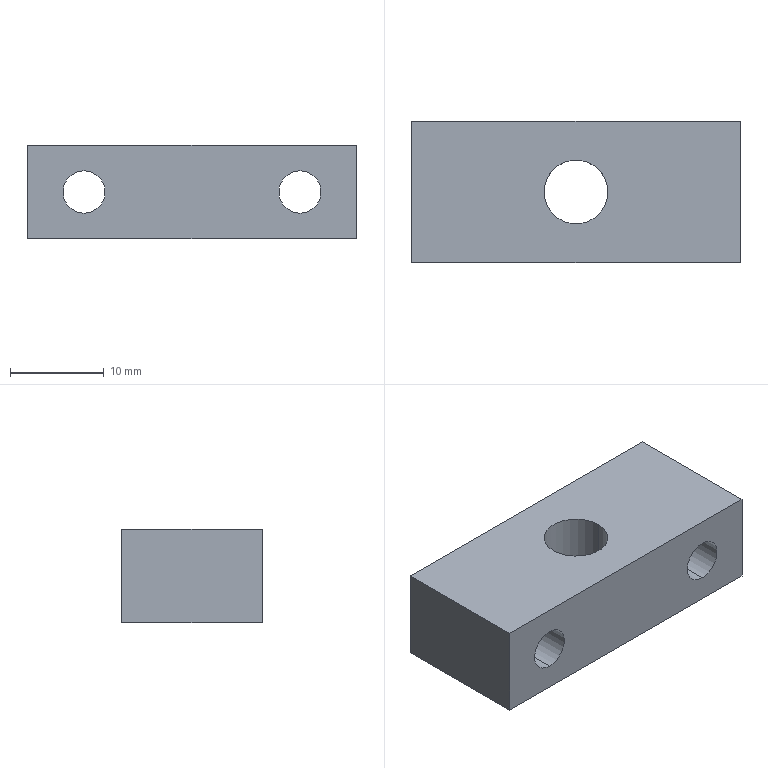Part | STEP file | Adjusting block | 1 solid | 18 faces | box 35 x 15 x 10 mm | volume 4094 mm3 | cylinder 10 | plane 8 | commonest cylinder face diameters 4.5 x4 8 x4 6.8 x2
STEP:
#1=CARTESIAN_POINT('',(0.,0.,0.));
#2=DIRECTION('',(0.,0.,1.));
#3=DIRECTION('',(1.,0.,0.));
#4=AXIS2_PLACEMENT_3D('',#1,#2,#3);
#5=CARTESIAN_POINT('',(3.4,0.,0.));
#6=VERTEX_POINT('',#5);
#7=CARTESIAN_POINT('',(3.4,0.,10.));
#8=VERTEX_POINT('',#7);
#9=CARTESIAN_POINT('',(3.4,0.,10.));
#10=DIRECTION('',(0.,0.,1.));
#11=VECTOR('',#10,1.);
#12=LINE('',#9,#11);
#13=CARTESIAN_POINT('',(0.,0.,10.));
#14=DIRECTION('',(0.,0.,1.));
#15=DIRECTION('',(1.,0.,0.));
#16=AXIS2_PLACEMENT_3D('',#13,#14,#15);
#17=CYLINDRICAL_SURFACE('',#16,3.4);
#18=CARTESIAN_POINT('',(6.283,0.));
#19=DIRECTION('',(0.,1.));
#20=VECTOR('',#19,1.);
#21=LINE('',#18,#20);
#22=(GEOMETRIC_REPRESENTATION_CONTEXT(2)PARAMETRIC_REPRESENTATION_CONTEXT()REPRESENTATION_CONTEXT('',''));
#23=DEFINITIONAL_REPRESENTATION('',(#21),#22);
#24=PCURVE('',#17,#23);
#25=CARTESIAN_POINT('',(0.,0.,10.));
#26=DIRECTION('',(0.,0.,1.));
#27=DIRECTION('',(1.,0.,0.));
#28=AXIS2_PLACEMENT_3D('',#25,#26,#27);
#29=CYLINDRICAL_SURFACE('',#28,3.4);
#30=CARTESIAN_POINT('',(0.,0.));
#31=DIRECTION('',(0.,1.));
#32=VECTOR('',#31,1.);
#33=LINE('',#30,#32);
#34=(GEOMETRIC_REPRESENTATION_CONTEXT(2)PARAMETRIC_REPRESENTATION_CONTEXT()REPRESENTATION_CONTEXT('',''));
#35=DEFINITIONAL_REPRESENTATION('',(#33),#34);
#36=PCURVE('',#29,#35);
#37=SURFACE_CURVE('',#12,(#24,#36),.PCURVE_S1.);
#38=EDGE_CURVE('',#6,#8,#37,.T.);
#39=ORIENTED_EDGE('',*,*,#38,.T.);
#40=CARTESIAN_POINT('',(-3.4,0.,10.));
#41=VERTEX_POINT('',#40);
#42=CARTESIAN_POINT('',(0.,0.,10.));
#43=DIRECTION('',(0.,0.,-1.));
#44=DIRECTION('',(1.,0.,0.));
#45=AXIS2_PLACEMENT_3D('',#42,#43,#44);
#46=CIRCLE('',#45,3.4);
#47=CARTESIAN_POINT('',(6.283,0.));
#48=DIRECTION('',(-1.,0.));
#49=VECTOR('',#48,1.);
#50=LINE('',#47,#49);
#51=(GEOMETRIC_REPRESENTATION_CONTEXT(2)PARAMETRIC_REPRESENTATION_CONTEXT()REPRESENTATION_CONTEXT('',''));
#52=DEFINITIONAL_REPRESENTATION('',(#50),#51);
#53=PCURVE('',#17,#52);
#54=CARTESIAN_POINT('',(0.,0.,10.));
#55=DIRECTION('',(0.,0.,1.));
#56=DIRECTION('',(1.,0.,0.));
#57=AXIS2_PLACEMENT_3D('',#54,#55,#56);
#58=PLANE('',#57);
#59=CARTESIAN_POINT('',(3.4,0.));
#60=CARTESIAN_POINT('',(3.4,-5.889));
#61=CARTESIAN_POINT('',(-1.7,-2.944));
#62=CARTESIAN_POINT('',(-6.8,0.));
#63=CARTESIAN_POINT('',(-1.7,2.944));
#64=CARTESIAN_POINT('',(3.4,5.889));
#65=CARTESIAN_POINT('',(3.4,0.));
#66=(BOUNDED_CURVE()B_SPLINE_CURVE(2,(#59,#60,#61,#62,#63,#64,#65),.UNSPECIFIED.,.T.,.F.)B_SPLINE_CURVE_WITH_KNOTS((1,2,2,2,2,1),(-2.094,0.,2.094,4.189,6.283,8.378),.UNSPECIFIED.)CURVE()GEOMETRIC_REPRESENTATION_ITEM()RATIONAL_B_SPLINE_CURVE((1.,0.5,1.,0.5,1.,0.5,1.))REPRESENTATION_ITEM(''));
#67=(GEOMETRIC_REPRESENTATION_CONTEXT(2)PARAMETRIC_REPRESENTATION_CONTEXT()REPRESENTATION_CONTEXT('',''));
#68=DEFINITIONAL_REPRESENTATION('',(#66),#67);
#69=PCURVE('',#58,#68);
#70=SURFACE_CURVE('',#46,(#53,#69),.PCURVE_S1.);
#71=EDGE_CURVE('',#8,#41,#70,.T.);
#72=ORIENTED_EDGE('',*,*,#71,.T.);
#73=CARTESIAN_POINT('',(-3.4,0.,0.));
#74=VERTEX_POINT('',#73);
#75=CARTESIAN_POINT('',(-3.4,0.,10.));
#76=DIRECTION('',(0.,0.,1.));
#77=VECTOR('',#76,1.);
#78=LINE('',#75,#77);
#79=CARTESIAN_POINT('',(3.142,0.));
#80=DIRECTION('',(0.,1.));
#81=VECTOR('',#80,1.);
#82=LINE('',#79,#81);
#83=(GEOMETRIC_REPRESENTATION_CONTEXT(2)PARAMETRIC_REPRESENTATION_CONTEXT()REPRESENTATION_CONTEXT('',''));
#84=DEFINITIONAL_REPRESENTATION('',(#82),#83);
#85=PCURVE('',#17,#84);
#86=CARTESIAN_POINT('',(3.142,0.));
#87=DIRECTION('',(0.,1.));
#88=VECTOR('',#87,1.);
#89=LINE('',#86,#88);
#90=(GEOMETRIC_REPRESENTATION_CONTEXT(2)PARAMETRIC_REPRESENTATION_CONTEXT()REPRESENTATION_CONTEXT('',''));
#91=DEFINITIONAL_REPRESENTATION('',(#89),#90);
#92=PCURVE('',#29,#91);
#93=SURFACE_CURVE('',#78,(#85,#92),.PCURVE_S1.);
#94=EDGE_CURVE('',#74,#41,#93,.T.);
#95=ORIENTED_EDGE('',*,*,#94,.F.);
#96=CARTESIAN_POINT('',(0.,0.,0.));
#97=DIRECTION('',(0.,0.,1.));
#98=DIRECTION('',(1.,0.,0.));
#99=AXIS2_PLACEMENT_3D('',#96,#97,#98);
#100=CIRCLE('',#99,3.4);
#101=CARTESIAN_POINT('',(0.,-10.));
#102=DIRECTION('',(1.,0.));
#103=VECTOR('',#102,1.);
#104=LINE('',#101,#103);
#105=(GEOMETRIC_REPRESENTATION_CONTEXT(2)PARAMETRIC_REPRESENTATION_CONTEXT()REPRESENTATION_CONTEXT('',''));
#106=DEFINITIONAL_REPRESENTATION('',(#104),#105);
#107=PCURVE('',#17,#106);
#108=CARTESIAN_POINT('',(0.,0.,0.));
#109=DIRECTION('',(0.,0.,1.));
#110=DIRECTION('',(1.,0.,0.));
#111=AXIS2_PLACEMENT_3D('',#108,#109,#110);
#112=PLANE('',#111);
#113=CARTESIAN_POINT('',(0.,0.));
#114=DIRECTION('',(1.,0.));
#115=AXIS2_PLACEMENT_2D('',#113,#114);
#116=CIRCLE('',#115,3.4);
#117=(GEOMETRIC_REPRESENTATION_CONTEXT(2)PARAMETRIC_REPRESENTATION_CONTEXT()REPRESENTATION_CONTEXT('',''));
#118=DEFINITIONAL_REPRESENTATION('',(#116),#117);
#119=PCURVE('',#112,#118);
#120=SURFACE_CURVE('',#100,(#107,#119),.PCURVE_S1.);
#121=EDGE_CURVE('',#74,#6,#120,.T.);
#122=ORIENTED_EDGE('',*,*,#121,.T.);
#123=EDGE_LOOP('',(#39,#72,#95,#122));
#124=FACE_BOUND('',#123,.F.);
#125=ADVANCED_FACE('',(#124),#17,.F.);
#126=CARTESIAN_POINT('',(11.5,-7.5,7.25));
#127=VERTEX_POINT('',#126);
#128=CARTESIAN_POINT('',(11.5,2.9,7.25));
#129=VERTEX_POINT('',#128);
#130=CARTESIAN_POINT('',(11.5,7.5,7.25));
#131=DIRECTION('',(0.,1.,0.));
#132=VECTOR('',#131,1.);
#133=LINE('',#130,#132);
#134=CARTESIAN_POINT('',(11.5,7.5,5.));
#135=DIRECTION('',(0.,1.,0.));
#136=DIRECTION('',(0.,0.,1.));
#137=AXIS2_PLACEMENT_3D('',#134,#135,#136);
#138=CYLINDRICAL_SURFACE('',#137,2.25);
#139=CARTESIAN_POINT('',(6.283,0.));
#140=DIRECTION('',(0.,1.));
#141=VECTOR('',#140,1.);
#142=LINE('',#139,#141);
#143=(GEOMETRIC_REPRESENTATION_CONTEXT(2)PARAMETRIC_REPRESENTATION_CONTEXT()REPRESENTATION_CONTEXT('',''));
#144=DEFINITIONAL_REPRESENTATION('',(#142),#143);
#145=PCURVE('',#138,#144);
#146=CARTESIAN_POINT('',(11.5,7.5,5.));
#147=DIRECTION('',(0.,1.,0.));
#148=DIRECTION('',(0.,0.,1.));
#149=AXIS2_PLACEMENT_3D('',#146,#147,#148);
#150=CYLINDRICAL_SURFACE('',#149,2.25);
#151=CARTESIAN_POINT('',(0.,0.));
#152=DIRECTION('',(0.,1.));
#153=VECTOR('',#152,1.);
#154=LINE('',#151,#153);
#155=(GEOMETRIC_REPRESENTATION_CONTEXT(2)PARAMETRIC_REPRESENTATION_CONTEXT()REPRESENTATION_CONTEXT('',''));
#156=DEFINITIONAL_REPRESENTATION('',(#154),#155);
#157=PCURVE('',#150,#156);
#158=SURFACE_CURVE('',#133,(#145,#157),.PCURVE_S1.);
#159=EDGE_CURVE('',#127,#129,#158,.T.);
#160=ORIENTED_EDGE('',*,*,#159,.T.);
#161=CARTESIAN_POINT('',(11.5,2.9,2.75));
#162=VERTEX_POINT('',#161);
#163=CARTESIAN_POINT('',(11.5,2.9,5.));
#164=DIRECTION('',(0.,-1.,0.));
#165=DIRECTION('',(0.,0.,1.));
#166=AXIS2_PLACEMENT_3D('',#163,#164,#165);
#167=CIRCLE('',#166,2.25);
#168=CARTESIAN_POINT('',(6.283,-4.6));
#169=DIRECTION('',(-1.,0.));
#170=VECTOR('',#169,1.);
#171=LINE('',#168,#170);
#172=(GEOMETRIC_REPRESENTATION_CONTEXT(2)PARAMETRIC_REPRESENTATION_CONTEXT()REPRESENTATION_CONTEXT('',''));
#173=DEFINITIONAL_REPRESENTATION('',(#171),#172);
#174=PCURVE('',#138,#173);
#175=CARTESIAN_POINT('',(13.75,2.9,5.));
#176=DIRECTION('',(0.,-1.,0.));
#177=DIRECTION('',(0.,0.,-1.));
#178=AXIS2_PLACEMENT_3D('',#175,#176,#177);
#179=PLANE('',#178);
#180=CARTESIAN_POINT('',(0.,-2.25));
#181=DIRECTION('',(-1.,0.));
#182=AXIS2_PLACEMENT_2D('',#180,#181);
#183=CIRCLE('',#182,2.25);
#184=(GEOMETRIC_REPRESENTATION_CONTEXT(2)PARAMETRIC_REPRESENTATION_CONTEXT()REPRESENTATION_CONTEXT('',''));
#185=DEFINITIONAL_REPRESENTATION('',(#183),#184);
#186=PCURVE('',#179,#185);
#187=SURFACE_CURVE('',#167,(#174,#186),.PCURVE_S1.);
#188=EDGE_CURVE('',#129,#162,#187,.T.);
#189=ORIENTED_EDGE('',*,*,#188,.T.);
#190=CARTESIAN_POINT('',(11.5,-7.5,2.75));
#191=VERTEX_POINT('',#190);
#192=CARTESIAN_POINT('',(11.5,7.5,2.75));
#193=DIRECTION('',(0.,1.,0.));
#194=VECTOR('',#193,1.);
#195=LINE('',#192,#194);
#196=CARTESIAN_POINT('',(3.142,0.));
#197=DIRECTION('',(0.,1.));
#198=VECTOR('',#197,1.);
#199=LINE('',#196,#198);
#200=(GEOMETRIC_REPRESENTATION_CONTEXT(2)PARAMETRIC_REPRESENTATION_CONTEXT()REPRESENTATION_CONTEXT('',''));
#201=DEFINITIONAL_REPRESENTATION('',(#199),#200);
#202=PCURVE('',#138,#201);
#203=CARTESIAN_POINT('',(3.142,0.));
#204=DIRECTION('',(0.,1.));
#205=VECTOR('',#204,1.);
#206=LINE('',#203,#205);
#207=(GEOMETRIC_REPRESENTATION_CONTEXT(2)PARAMETRIC_REPRESENTATION_CONTEXT()REPRESENTATION_CONTEXT('',''));
#208=DEFINITIONAL_REPRESENTATION('',(#206),#207);
#209=PCURVE('',#150,#208);
#210=SURFACE_CURVE('',#195,(#202,#209),.PCURVE_S1.);
#211=EDGE_CURVE('',#191,#162,#210,.T.);
#212=ORIENTED_EDGE('',*,*,#211,.F.);
#213=CARTESIAN_POINT('',(11.5,-7.5,5.));
#214=DIRECTION('',(0.,-1.,0.));
#215=DIRECTION('',(0.,0.,1.));
#216=AXIS2_PLACEMENT_3D('',#213,#214,#215);
#217=CIRCLE('',#216,2.25);
#218=CARTESIAN_POINT('',(6.283,-15.));
#219=DIRECTION('',(-1.,0.));
#220=VECTOR('',#219,1.);
#221=LINE('',#218,#220);
#222=(GEOMETRIC_REPRESENTATION_CONTEXT(2)PARAMETRIC_REPRESENTATION_CONTEXT()REPRESENTATION_CONTEXT('',''));
#223=DEFINITIONAL_REPRESENTATION('',(#221),#222);
#224=PCURVE('',#138,#223);
#225=CARTESIAN_POINT('',(-17.5,-7.5,10.));
#226=DIRECTION('',(0.,1.,0.));
#227=DIRECTION('',(0.,0.,1.));
#228=AXIS2_PLACEMENT_3D('',#225,#226,#227);
#229=PLANE('',#228);
#230=CARTESIAN_POINT('',(-2.75,29.));
#231=CARTESIAN_POINT('',(-2.75,25.103));
#232=CARTESIAN_POINT('',(-6.125,27.051));
#233=CARTESIAN_POINT('',(-9.5,29.));
#234=CARTESIAN_POINT('',(-6.125,30.949));
#235=CARTESIAN_POINT('',(-2.75,32.897));
#236=CARTESIAN_POINT('',(-2.75,29.));
#237=(BOUNDED_CURVE()B_SPLINE_CURVE(2,(#230,#231,#232,#233,#234,#235,#236),.UNSPECIFIED.,.T.,.F.)B_SPLINE_CURVE_WITH_KNOTS((1,2,2,2,2,1),(-2.094,0.,2.094,4.189,6.283,8.378),.UNSPECIFIED.)CURVE()GEOMETRIC_REPRESENTATION_ITEM()RATIONAL_B_SPLINE_CURVE((1.,0.5,1.,0.5,1.,0.5,1.))REPRESENTATION_ITEM(''));
#238=(GEOMETRIC_REPRESENTATION_CONTEXT(2)PARAMETRIC_REPRESENTATION_CONTEXT()REPRESENTATION_CONTEXT('',''));
#239=DEFINITIONAL_REPRESENTATION('',(#237),#238);
#240=PCURVE('',#229,#239);
#241=SURFACE_CURVE('',#217,(#224,#240),.PCURVE_S1.);
#242=EDGE_CURVE('',#127,#191,#241,.T.);
#243=ORIENTED_EDGE('',*,*,#242,.F.);
#244=EDGE_LOOP('',(#160,#189,#212,#243));
#245=FACE_BOUND('',#244,.F.);
#246=ADVANCED_FACE('',(#245),#138,.F.);
#247=CARTESIAN_POINT('',(-11.5,-7.5,7.25));
#248=VERTEX_POINT('',#247);
#249=CARTESIAN_POINT('',(-11.5,2.9,7.25));
#250=VERTEX_POINT('',#249);
#251=CARTESIAN_POINT('',(-11.5,7.5,7.25));
#252=DIRECTION('',(0.,1.,0.));
#253=VECTOR('',#252,1.);
#254=LINE('',#251,#253);
#255=CARTESIAN_POINT('',(-11.5,7.5,5.));
#256=DIRECTION('',(0.,1.,0.));
#257=DIRECTION('',(0.,0.,1.));
#258=AXIS2_PLACEMENT_3D('',#255,#256,#257);
#259=CYLINDRICAL_SURFACE('',#258,2.25);
#260=CARTESIAN_POINT('',(6.283,0.));
#261=DIRECTION('',(0.,1.));
#262=VECTOR('',#261,1.);
#263=LINE('',#260,#262);
#264=(GEOMETRIC_REPRESENTATION_CONTEXT(2)PARAMETRIC_REPRESENTATION_CONTEXT()REPRESENTATION_CONTEXT('',''));
#265=DEFINITIONAL_REPRESENTATION('',(#263),#264);
#266=PCURVE('',#259,#265);
#267=CARTESIAN_POINT('',(-11.5,7.5,5.));
#268=DIRECTION('',(0.,1.,0.));
#269=DIRECTION('',(0.,0.,1.));
#270=AXIS2_PLACEMENT_3D('',#267,#268,#269);
#271=CYLINDRICAL_SURFACE('',#270,2.25);
#272=CARTESIAN_POINT('',(0.,0.));
#273=DIRECTION('',(0.,1.));
#274=VECTOR('',#273,1.);
#275=LINE('',#272,#274);
#276=(GEOMETRIC_REPRESENTATION_CONTEXT(2)PARAMETRIC_REPRESENTATION_CONTEXT()REPRESENTATION_CONTEXT('',''));
#277=DEFINITIONAL_REPRESENTATION('',(#275),#276);
#278=PCURVE('',#271,#277);
#279=SURFACE_CURVE('',#254,(#266,#278),.PCURVE_S1.);
#280=EDGE_CURVE('',#248,#250,#279,.T.);
#281=ORIENTED_EDGE('',*,*,#280,.T.);
#282=CARTESIAN_POINT('',(-11.5,2.9,2.75));
#283=VERTEX_POINT('',#282);
#284=CARTESIAN_POINT('',(-11.5,2.9,5.));
#285=DIRECTION('',(0.,-1.,0.));
#286=DIRECTION('',(0.,0.,1.));
#287=AXIS2_PLACEMENT_3D('',#284,#285,#286);
#288=CIRCLE('',#287,2.25);
#289=CARTESIAN_POINT('',(6.283,-4.6));
#290=DIRECTION('',(-1.,0.));
#291=VECTOR('',#290,1.);
#292=LINE('',#289,#291);
#293=(GEOMETRIC_REPRESENTATION_CONTEXT(2)PARAMETRIC_REPRESENTATION_CONTEXT()REPRESENTATION_CONTEXT('',''));
#294=DEFINITIONAL_REPRESENTATION('',(#292),#293);
#295=PCURVE('',#259,#294);
#296=CARTESIAN_POINT('',(-9.25,2.9,5.));
#297=DIRECTION('',(0.,-1.,0.));
#298=DIRECTION('',(0.,0.,-1.));
#299=AXIS2_PLACEMENT_3D('',#296,#297,#298);
#300=PLANE('',#299);
#301=CARTESIAN_POINT('',(0.,-2.25));
#302=DIRECTION('',(-1.,0.));
#303=AXIS2_PLACEMENT_2D('',#301,#302);
#304=CIRCLE('',#303,2.25);
#305=(GEOMETRIC_REPRESENTATION_CONTEXT(2)PARAMETRIC_REPRESENTATION_CONTEXT()REPRESENTATION_CONTEXT('',''));
#306=DEFINITIONAL_REPRESENTATION('',(#304),#305);
#307=PCURVE('',#300,#306);
#308=SURFACE_CURVE('',#288,(#295,#307),.PCURVE_S1.);
#309=EDGE_CURVE('',#250,#283,#308,.T.);
#310=ORIENTED_EDGE('',*,*,#309,.T.);
#311=CARTESIAN_POINT('',(-11.5,-7.5,2.75));
#312=VERTEX_POINT('',#311);
#313=CARTESIAN_POINT('',(-11.5,7.5,2.75));
#314=DIRECTION('',(0.,1.,0.));
#315=VECTOR('',#314,1.);
#316=LINE('',#313,#315);
#317=CARTESIAN_POINT('',(3.142,0.));
#318=DIRECTION('',(0.,1.));
#319=VECTOR('',#318,1.);
#320=LINE('',#317,#319);
#321=(GEOMETRIC_REPRESENTATION_CONTEXT(2)PARAMETRIC_REPRESENTATION_CONTEXT()REPRESENTATION_CONTEXT('',''));
#322=DEFINITIONAL_REPRESENTATION('',(#320),#321);
#323=PCURVE('',#259,#322);
#324=CARTESIAN_POINT('',(3.142,0.));
#325=DIRECTION('',(0.,1.));
#326=VECTOR('',#325,1.);
#327=LINE('',#324,#326);
#328=(GEOMETRIC_REPRESENTATION_CONTEXT(2)PARAMETRIC_REPRESENTATION_CONTEXT()REPRESENTATION_CONTEXT('',''));
#329=DEFINITIONAL_REPRESENTATION('',(#327),#328);
#330=PCURVE('',#271,#329);
#331=SURFACE_CURVE('',#316,(#323,#330),.PCURVE_S1.);
#332=EDGE_CURVE('',#312,#283,#331,.T.);
#333=ORIENTED_EDGE('',*,*,#332,.F.);
#334=CARTESIAN_POINT('',(-11.5,-7.5,5.));
#335=DIRECTION('',(0.,-1.,0.));
#336=DIRECTION('',(0.,0.,1.));
#337=AXIS2_PLACEMENT_3D('',#334,#335,#336);
#338=CIRCLE('',#337,2.25);
#339=CARTESIAN_POINT('',(6.283,-15.));
#340=DIRECTION('',(-1.,0.));
#341=VECTOR('',#340,1.);
#342=LINE('',#339,#341);
#343=(GEOMETRIC_REPRESENTATION_CONTEXT(2)PARAMETRIC_REPRESENTATION_CONTEXT()REPRESENTATION_CONTEXT('',''));
#344=DEFINITIONAL_REPRESENTATION('',(#342),#343);
#345=PCURVE('',#259,#344);
#346=CARTESIAN_POINT('',(-2.75,6.));
#347=CARTESIAN_POINT('',(-2.75,2.103));
#348=CARTESIAN_POINT('',(-6.125,4.051));
#349=CARTESIAN_POINT('',(-9.5,6.));
#350=CARTESIAN_POINT('',(-6.125,7.949));
#351=CARTESIAN_POINT('',(-2.75,9.897));
#352=CARTESIAN_POINT('',(-2.75,6.));
#353=(BOUNDED_CURVE()B_SPLINE_CURVE(2,(#346,#347,#348,#349,#350,#351,#352),.UNSPECIFIED.,.T.,.F.)B_SPLINE_CURVE_WITH_KNOTS((1,2,2,2,2,1),(-2.094,0.,2.094,4.189,6.283,8.378),.UNSPECIFIED.)CURVE()GEOMETRIC_REPRESENTATION_ITEM()RATIONAL_B_SPLINE_CURVE((1.,0.5,1.,0.5,1.,0.5,1.))REPRESENTATION_ITEM(''));
#354=(GEOMETRIC_REPRESENTATION_CONTEXT(2)PARAMETRIC_REPRESENTATION_CONTEXT()REPRESENTATION_CONTEXT('',''));
#355=DEFINITIONAL_REPRESENTATION('',(#353),#354);
#356=PCURVE('',#229,#355);
#357=SURFACE_CURVE('',#338,(#345,#356),.PCURVE_S1.);
#358=EDGE_CURVE('',#248,#312,#357,.T.);
#359=ORIENTED_EDGE('',*,*,#358,.F.);
#360=EDGE_LOOP('',(#281,#310,#333,#359));
#361=FACE_BOUND('',#360,.F.);
#362=ADVANCED_FACE('',(#361),#259,.F.);
#363=CARTESIAN_POINT('',(11.5,2.9,9.));
#364=VERTEX_POINT('',#363);
#365=CARTESIAN_POINT('',(11.5,7.5,9.));
#366=VERTEX_POINT('',#365);
#367=CARTESIAN_POINT('',(11.5,7.5,9.));
#368=DIRECTION('',(0.,1.,0.));
#369=VECTOR('',#368,1.);
#370=LINE('',#367,#369);
#371=CARTESIAN_POINT('',(11.5,7.5,5.));
#372=DIRECTION('',(0.,1.,0.));
#373=DIRECTION('',(0.,0.,1.));
#374=AXIS2_PLACEMENT_3D('',#371,#372,#373);
#375=CYLINDRICAL_SURFACE('',#374,4.);
#376=CARTESIAN_POINT('',(6.283,0.));
#377=DIRECTION('',(0.,1.));
#378=VECTOR('',#377,1.);
#379=LINE('',#376,#378);
#380=(GEOMETRIC_REPRESENTATION_CONTEXT(2)PARAMETRIC_REPRESENTATION_CONTEXT()REPRESENTATION_CONTEXT('',''));
#381=DEFINITIONAL_REPRESENTATION('',(#379),#380);
#382=PCURVE('',#375,#381);
#383=CARTESIAN_POINT('',(11.5,7.5,5.));
#384=DIRECTION('',(0.,1.,0.));
#385=DIRECTION('',(0.,0.,1.));
#386=AXIS2_PLACEMENT_3D('',#383,#384,#385);
#387=CYLINDRICAL_SURFACE('',#386,4.);
#388=CARTESIAN_POINT('',(0.,0.));
#389=DIRECTION('',(0.,1.));
#390=VECTOR('',#389,1.);
#391=LINE('',#388,#390);
#392=(GEOMETRIC_REPRESENTATION_CONTEXT(2)PARAMETRIC_REPRESENTATION_CONTEXT()REPRESENTATION_CONTEXT('',''));
#393=DEFINITIONAL_REPRESENTATION('',(#391),#392);
#394=PCURVE('',#387,#393);
#395=SURFACE_CURVE('',#370,(#382,#394),.PCURVE_S1.);
#396=EDGE_CURVE('',#364,#366,#395,.T.);
#397=ORIENTED_EDGE('',*,*,#396,.T.);
#398=CARTESIAN_POINT('',(11.5,7.5,1.));
#399=VERTEX_POINT('',#398);
#400=CARTESIAN_POINT('',(11.5,7.5,5.));
#401=DIRECTION('',(0.,1.,0.));
#402=DIRECTION('',(0.,0.,1.));
#403=AXIS2_PLACEMENT_3D('',#400,#401,#402);
#404=CIRCLE('',#403,4.);
#405=CARTESIAN_POINT('',(0.,0.));
#406=DIRECTION('',(1.,0.));
#407=VECTOR('',#406,1.);
#408=LINE('',#405,#407);
#409=(GEOMETRIC_REPRESENTATION_CONTEXT(2)PARAMETRIC_REPRESENTATION_CONTEXT()REPRESENTATION_CONTEXT('',''));
#410=DEFINITIONAL_REPRESENTATION('',(#408),#409);
#411=PCURVE('',#375,#410);
#412=CARTESIAN_POINT('',(-17.5,7.5,10.));
#413=DIRECTION('',(0.,-1.,0.));
#414=DIRECTION('',(0.,0.,-1.));
#415=AXIS2_PLACEMENT_3D('',#412,#413,#414);
#416=PLANE('',#415);
#417=CARTESIAN_POINT('',(1.,29.));
#418=CARTESIAN_POINT('',(1.,35.928));
#419=CARTESIAN_POINT('',(7.,32.464));
#420=CARTESIAN_POINT('',(13.,29.));
#421=CARTESIAN_POINT('',(7.,25.536));
#422=CARTESIAN_POINT('',(1.,22.072));
#423=CARTESIAN_POINT('',(1.,29.));
#424=(BOUNDED_CURVE()B_SPLINE_CURVE(2,(#417,#418,#419,#420,#421,#422,#423),.UNSPECIFIED.,.T.,.F.)B_SPLINE_CURVE_WITH_KNOTS((1,2,2,2,2,1),(-2.094,0.,2.094,4.189,6.283,8.378),.UNSPECIFIED.)CURVE()GEOMETRIC_REPRESENTATION_ITEM()RATIONAL_B_SPLINE_CURVE((1.,0.5,1.,0.5,1.,0.5,1.))REPRESENTATION_ITEM(''));
#425=(GEOMETRIC_REPRESENTATION_CONTEXT(2)PARAMETRIC_REPRESENTATION_CONTEXT()REPRESENTATION_CONTEXT('',''));
#426=DEFINITIONAL_REPRESENTATION('',(#424),#425);
#427=PCURVE('',#416,#426);
#428=SURFACE_CURVE('',#404,(#411,#427),.PCURVE_S1.);
#429=EDGE_CURVE('',#399,#366,#428,.T.);
#430=ORIENTED_EDGE('',*,*,#429,.F.);
#431=CARTESIAN_POINT('',(11.5,2.9,1.));
#432=VERTEX_POINT('',#431);
#433=CARTESIAN_POINT('',(11.5,7.5,1.));
#434=DIRECTION('',(0.,1.,0.));
#435=VECTOR('',#434,1.);
#436=LINE('',#433,#435);
#437=CARTESIAN_POINT('',(3.142,0.));
#438=DIRECTION('',(0.,1.));
#439=VECTOR('',#438,1.);
#440=LINE('',#437,#439);
#441=(GEOMETRIC_REPRESENTATION_CONTEXT(2)PARAMETRIC_REPRESENTATION_CONTEXT()REPRESENTATION_CONTEXT('',''));
#442=DEFINITIONAL_REPRESENTATION('',(#440),#441);
#443=PCURVE('',#375,#442);
#444=CARTESIAN_POINT('',(3.142,0.));
#445=DIRECTION('',(0.,1.));
#446=VECTOR('',#445,1.);
#447=LINE('',#444,#446);
#448=(GEOMETRIC_REPRESENTATION_CONTEXT(2)PARAMETRIC_REPRESENTATION_CONTEXT()REPRESENTATION_CONTEXT('',''));
#449=DEFINITIONAL_REPRESENTATION('',(#447),#448);
#450=PCURVE('',#387,#449);
#451=SURFACE_CURVE('',#436,(#443,#450),.PCURVE_S1.);
#452=EDGE_CURVE('',#432,#399,#451,.T.);
#453=ORIENTED_EDGE('',*,*,#452,.F.);
#454=CARTESIAN_POINT('',(11.5,2.9,5.));
#455=DIRECTION('',(0.,1.,0.));
#456=DIRECTION('',(0.,0.,1.));
#457=AXIS2_PLACEMENT_3D('',#454,#455,#456);
#458=CIRCLE('',#457,4.);
#459=CARTESIAN_POINT('',(0.,-4.6));
#460=DIRECTION('',(1.,0.));
#461=VECTOR('',#460,1.);
#462=LINE('',#459,#461);
#463=(GEOMETRIC_REPRESENTATION_CONTEXT(2)PARAMETRIC_REPRESENTATION_CONTEXT()REPRESENTATION_CONTEXT('',''));
#464=DEFINITIONAL_REPRESENTATION('',(#462),#463);
#465=PCURVE('',#375,#464);
#466=CARTESIAN_POINT('',(-4.,-2.25));
#467=CARTESIAN_POINT('',(-4.,4.678));
#468=CARTESIAN_POINT('',(2.,1.214));
#469=CARTESIAN_POINT('',(8.,-2.25));
#470=CARTESIAN_POINT('',(2.,-5.714));
#471=CARTESIAN_POINT('',(-4.,-9.178));
#472=CARTESIAN_POINT('',(-4.,-2.25));
#473=(BOUNDED_CURVE()B_SPLINE_CURVE(2,(#466,#467,#468,#469,#470,#471,#472),.UNSPECIFIED.,.T.,.F.)B_SPLINE_CURVE_WITH_KNOTS((1,2,2,2,2,1),(-2.094,0.,2.094,4.189,6.283,8.378),.UNSPECIFIED.)CURVE()GEOMETRIC_REPRESENTATION_ITEM()RATIONAL_B_SPLINE_CURVE((1.,0.5,1.,0.5,1.,0.5,1.))REPRESENTATION_ITEM(''));
#474=(GEOMETRIC_REPRESENTATION_CONTEXT(2)PARAMETRIC_REPRESENTATION_CONTEXT()REPRESENTATION_CONTEXT('',''));
#475=DEFINITIONAL_REPRESENTATION('',(#473),#474);
#476=PCURVE('',#179,#475);
#477=SURFACE_CURVE('',#458,(#465,#476),.PCURVE_S1.);
#478=EDGE_CURVE('',#432,#364,#477,.T.);
#479=ORIENTED_EDGE('',*,*,#478,.T.);
#480=EDGE_LOOP('',(#397,#430,#453,#479));
#481=FACE_BOUND('',#480,.F.);
#482=ADVANCED_FACE('',(#481),#375,.F.);
#483=CARTESIAN_POINT('',(-11.5,2.9,9.));
#484=VERTEX_POINT('',#483);
#485=CARTESIAN_POINT('',(-11.5,7.5,9.));
#486=VERTEX_POINT('',#485);
#487=CARTESIAN_POINT('',(-11.5,7.5,9.));
#488=DIRECTION('',(0.,1.,0.));
#489=VECTOR('',#488,1.);
#490=LINE('',#487,#489);
#491=CARTESIAN_POINT('',(-11.5,7.5,5.));
#492=DIRECTION('',(0.,1.,0.));
#493=DIRECTION('',(0.,0.,1.));
#494=AXIS2_PLACEMENT_3D('',#491,#492,#493);
#495=CYLINDRICAL_SURFACE('',#494,4.);
#496=CARTESIAN_POINT('',(6.283,0.));
#497=DIRECTION('',(0.,1.));
#498=VECTOR('',#497,1.);
#499=LINE('',#496,#498);
#500=(GEOMETRIC_REPRESENTATION_CONTEXT(2)PARAMETRIC_REPRESENTATION_CONTEXT()REPRESENTATION_CONTEXT('',''));
#501=DEFINITIONAL_REPRESENTATION('',(#499),#500);
#502=PCURVE('',#495,#501);
#503=CARTESIAN_POINT('',(-11.5,7.5,5.));
#504=DIRECTION('',(0.,1.,0.));
#505=DIRECTION('',(0.,0.,1.));
#506=AXIS2_PLACEMENT_3D('',#503,#504,#505);
#507=CYLINDRICAL_SURFACE('',#506,4.);
#508=CARTESIAN_POINT('',(0.,0.));
#509=DIRECTION('',(0.,1.));
#510=VECTOR('',#509,1.);
#511=LINE('',#508,#510);
#512=(GEOMETRIC_REPRESENTATION_CONTEXT(2)PARAMETRIC_REPRESENTATION_CONTEXT()REPRESENTATION_CONTEXT('',''));
#513=DEFINITIONAL_REPRESENTATION('',(#511),#512);
#514=PCURVE('',#507,#513);
#515=SURFACE_CURVE('',#490,(#502,#514),.PCURVE_S1.);
#516=EDGE_CURVE('',#484,#486,#515,.T.);
#517=ORIENTED_EDGE('',*,*,#516,.T.);
#518=CARTESIAN_POINT('',(-11.5,7.5,1.));
#519=VERTEX_POINT('',#518);
#520=CARTESIAN_POINT('',(-11.5,7.5,5.));
#521=DIRECTION('',(0.,1.,0.));
#522=DIRECTION('',(0.,0.,1.));
#523=AXIS2_PLACEMENT_3D('',#520,#521,#522);
#524=CIRCLE('',#523,4.);
#525=CARTESIAN_POINT('',(0.,0.));
#526=DIRECTION('',(1.,0.));
#527=VECTOR('',#526,1.);
#528=LINE('',#525,#527);
#529=(GEOMETRIC_REPRESENTATION_CONTEXT(2)PARAMETRIC_REPRESENTATION_CONTEXT()REPRESENTATION_CONTEXT('',''));
#530=DEFINITIONAL_REPRESENTATION('',(#528),#529);
#531=PCURVE('',#495,#530);
#532=CARTESIAN_POINT('',(1.,6.));
#533=CARTESIAN_POINT('',(1.,12.928));
#534=CARTESIAN_POINT('',(7.,9.464));
#535=CARTESIAN_POINT('',(13.,6.));
#536=CARTESIAN_POINT('',(7.,2.536));
#537=CARTESIAN_POINT('',(1.,-0.9282));
#538=CARTESIAN_POINT('',(1.,6.));
#539=(BOUNDED_CURVE()B_SPLINE_CURVE(2,(#532,#533,#534,#535,#536,#537,#538),.UNSPECIFIED.,.T.,.F.)B_SPLINE_CURVE_WITH_KNOTS((1,2,2,2,2,1),(-2.094,0.,2.094,4.189,6.283,8.378),.UNSPECIFIED.)CURVE()GEOMETRIC_REPRESENTATION_ITEM()RATIONAL_B_SPLINE_CURVE((1.,0.5,1.,0.5,1.,0.5,1.))REPRESENTATION_ITEM(''));
#540=(GEOMETRIC_REPRESENTATION_CONTEXT(2)PARAMETRIC_REPRESENTATION_CONTEXT()REPRESENTATION_CONTEXT('',''));
#541=DEFINITIONAL_REPRESENTATION('',(#539),#540);
#542=PCURVE('',#416,#541);
#543=SURFACE_CURVE('',#524,(#531,#542),.PCURVE_S1.);
#544=EDGE_CURVE('',#519,#486,#543,.T.);
#545=ORIENTED_EDGE('',*,*,#544,.F.);
#546=CARTESIAN_POINT('',(-11.5,2.9,1.));
#547=VERTEX_POINT('',#546);
#548=CARTESIAN_POINT('',(-11.5,7.5,1.));
#549=DIRECTION('',(0.,1.,0.));
#550=VECTOR('',#549,1.);
#551=LINE('',#548,#550);
#552=CARTESIAN_POINT('',(3.142,0.));
#553=DIRECTION('',(0.,1.));
#554=VECTOR('',#553,1.);
#555=LINE('',#552,#554);
#556=(GEOMETRIC_REPRESENTATION_CONTEXT(2)PARAMETRIC_REPRESENTATION_CONTEXT()REPRESENTATION_CONTEXT('',''));
#557=DEFINITIONAL_REPRESENTATION('',(#555),#556);
#558=PCURVE('',#495,#557);
#559=CARTESIAN_POINT('',(3.142,0.));
#560=DIRECTION('',(0.,1.));
#561=VECTOR('',#560,1.);
#562=LINE('',#559,#561);
#563=(GEOMETRIC_REPRESENTATION_CONTEXT(2)PARAMETRIC_REPRESENTATION_CONTEXT()REPRESENTATION_CONTEXT('',''));
#564=DEFINITIONAL_REPRESENTATION('',(#562),#563);
#565=PCURVE('',#507,#564);
#566=SURFACE_CURVE('',#551,(#558,#565),.PCURVE_S1.);
#567=EDGE_CURVE('',#547,#519,#566,.T.);
#568=ORIENTED_EDGE('',*,*,#567,.F.);
#569=CARTESIAN_POINT('',(-11.5,2.9,5.));
#570=DIRECTION('',(0.,1.,0.));
#571=DIRECTION('',(0.,0.,1.));
#572=AXIS2_PLACEMENT_3D('',#569,#570,#571);
#573=CIRCLE('',#572,4.);
#574=CARTESIAN_POINT('',(0.,-4.6));
#575=DIRECTION('',(1.,0.));
#576=VECTOR('',#575,1.);
#577=LINE('',#574,#576);
#578=(GEOMETRIC_REPRESENTATION_CONTEXT(2)PARAMETRIC_REPRESENTATION_CONTEXT()REPRESENTATION_CONTEXT('',''));
#579=DEFINITIONAL_REPRESENTATION('',(#577),#578);
#580=PCURVE('',#495,#579);
#581=CARTESIAN_POINT('',(-4.,-2.25));
#582=CARTESIAN_POINT('',(-4.,4.678));
#583=CARTESIAN_POINT('',(2.,1.214));
#584=CARTESIAN_POINT('',(8.,-2.25));
#585=CARTESIAN_POINT('',(2.,-5.714));
#586=CARTESIAN_POINT('',(-4.,-9.178));
#587=CARTESIAN_POINT('',(-4.,-2.25));
#588=(BOUNDED_CURVE()B_SPLINE_CURVE(2,(#581,#582,#583,#584,#585,#586,#587),.UNSPECIFIED.,.T.,.F.)B_SPLINE_CURVE_WITH_KNOTS((1,2,2,2,2,1),(-2.094,0.,2.094,4.189,6.283,8.378),.UNSPECIFIED.)CURVE()GEOMETRIC_REPRESENTATION_ITEM()RATIONAL_B_SPLINE_CURVE((1.,0.5,1.,0.5,1.,0.5,1.))REPRESENTATION_ITEM(''));
#589=(GEOMETRIC_REPRESENTATION_CONTEXT(2)PARAMETRIC_REPRESENTATION_CONTEXT()REPRESENTATION_CONTEXT('',''));
#590=DEFINITIONAL_REPRESENTATION('',(#588),#589);
#591=PCURVE('',#300,#590);
#592=SURFACE_CURVE('',#573,(#580,#591),.PCURVE_S1.);
#593=EDGE_CURVE('',#547,#484,#592,.T.);
#594=ORIENTED_EDGE('',*,*,#593,.T.);
#595=EDGE_LOOP('',(#517,#545,#568,#594));
#596=FACE_BOUND('',#595,.F.);
#597=ADVANCED_FACE('',(#596),#495,.F.);
#598=CARTESIAN_POINT('',(-17.5,7.5,10.));
#599=VERTEX_POINT('',#598);
#600=CARTESIAN_POINT('',(-17.5,-7.5,10.));
#601=VERTEX_POINT('',#600);
#602=CARTESIAN_POINT('',(-17.5,0.,10.));
#603=DIRECTION('',(0.,-1.,0.));
#604=VECTOR('',#603,1.);
#605=LINE('',#602,#604);
#606=CARTESIAN_POINT('',(-17.5,0.));
#607=DIRECTION('',(0.,-1.));
#608=VECTOR('',#607,1.);
#609=LINE('',#606,#608);
#610=(GEOMETRIC_REPRESENTATION_CONTEXT(2)PARAMETRIC_REPRESENTATION_CONTEXT()REPRESENTATION_CONTEXT('',''));
#611=DEFINITIONAL_REPRESENTATION('',(#609),#610);
#612=PCURVE('',#58,#611);
#613=CARTESIAN_POINT('',(-17.5,7.5,10.));
#614=DIRECTION('',(1.,0.,0.));
#615=DIRECTION('',(0.,0.,-1.));
#616=AXIS2_PLACEMENT_3D('',#613,#614,#615);
#617=PLANE('',#616);
#618=CARTESIAN_POINT('',(0.,-7.5));
#619=DIRECTION('',(0.,-1.));
#620=VECTOR('',#619,1.);
#621=LINE('',#618,#620);
#622=(GEOMETRIC_REPRESENTATION_CONTEXT(2)PARAMETRIC_REPRESENTATION_CONTEXT()REPRESENTATION_CONTEXT('',''));
#623=DEFINITIONAL_REPRESENTATION('',(#621),#622);
#624=PCURVE('',#617,#623);
#625=SURFACE_CURVE('',#605,(#612,#624),.PCURVE_S1.);
#626=EDGE_CURVE('',#599,#601,#625,.T.);
#627=ORIENTED_EDGE('',*,*,#626,.T.);
#628=CARTESIAN_POINT('',(17.5,-7.5,10.));
#629=VERTEX_POINT('',#628);
#630=CARTESIAN_POINT('',(0.,-7.5,10.));
#631=DIRECTION('',(1.,0.,0.));
#632=VECTOR('',#631,1.);
#633=LINE('',#630,#632);
#634=CARTESIAN_POINT('',(0.,-7.5));
#635=DIRECTION('',(1.,0.));
#636=VECTOR('',#635,1.);
#637=LINE('',#634,#636);
#638=(GEOMETRIC_REPRESENTATION_CONTEXT(2)PARAMETRIC_REPRESENTATION_CONTEXT()REPRESENTATION_CONTEXT('',''));
#639=DEFINITIONAL_REPRESENTATION('',(#637),#638);
#640=PCURVE('',#58,#639);
#641=CARTESIAN_POINT('',(0.,17.5));
#642=DIRECTION('',(0.,1.));
#643=VECTOR('',#642,1.);
#644=LINE('',#641,#643);
#645=(GEOMETRIC_REPRESENTATION_CONTEXT(2)PARAMETRIC_REPRESENTATION_CONTEXT()REPRESENTATION_CONTEXT('',''));
#646=DEFINITIONAL_REPRESENTATION('',(#644),#645);
#647=PCURVE('',#229,#646);
#648=SURFACE_CURVE('',#633,(#640,#647),.PCURVE_S1.);
#649=EDGE_CURVE('',#601,#629,#648,.T.);
#650=ORIENTED_EDGE('',*,*,#649,.T.);
#651=CARTESIAN_POINT('',(17.5,7.5,10.));
#652=VERTEX_POINT('',#651);
#653=CARTESIAN_POINT('',(17.5,0.,10.));
#654=DIRECTION('',(0.,1.,0.));
#655=VECTOR('',#654,1.);
#656=LINE('',#653,#655);
#657=CARTESIAN_POINT('',(17.5,0.));
#658=DIRECTION('',(0.,1.));
#659=VECTOR('',#658,1.);
#660=LINE('',#657,#659);
#661=(GEOMETRIC_REPRESENTATION_CONTEXT(2)PARAMETRIC_REPRESENTATION_CONTEXT()REPRESENTATION_CONTEXT('',''));
#662=DEFINITIONAL_REPRESENTATION('',(#660),#661);
#663=PCURVE('',#58,#662);
#664=CARTESIAN_POINT('',(17.5,7.5,10.));
#665=DIRECTION('',(-1.,0.,0.));
#666=DIRECTION('',(0.,0.,1.));
#667=AXIS2_PLACEMENT_3D('',#664,#665,#666);
#668=PLANE('',#667);
#669=CARTESIAN_POINT('',(0.,-7.5));
#670=DIRECTION('',(0.,1.));
#671=VECTOR('',#670,1.);
#672=LINE('',#669,#671);
#673=(GEOMETRIC_REPRESENTATION_CONTEXT(2)PARAMETRIC_REPRESENTATION_CONTEXT()REPRESENTATION_CONTEXT('',''));
#674=DEFINITIONAL_REPRESENTATION('',(#672),#673);
#675=PCURVE('',#668,#674);
#676=SURFACE_CURVE('',#656,(#663,#675),.PCURVE_S1.);
#677=EDGE_CURVE('',#629,#652,#676,.T.);
#678=ORIENTED_EDGE('',*,*,#677,.T.);
#679=CARTESIAN_POINT('',(0.,7.5,10.));
#680=DIRECTION('',(-1.,0.,0.));
#681=VECTOR('',#680,1.);
#682=LINE('',#679,#681);
#683=CARTESIAN_POINT('',(0.,7.5));
#684=DIRECTION('',(-1.,0.));
#685=VECTOR('',#684,1.);
#686=LINE('',#683,#685);
#687=(GEOMETRIC_REPRESENTATION_CONTEXT(2)PARAMETRIC_REPRESENTATION_CONTEXT()REPRESENTATION_CONTEXT('',''));
#688=DEFINITIONAL_REPRESENTATION('',(#686),#687);
#689=PCURVE('',#58,#688);
#690=CARTESIAN_POINT('',(0.,17.5));
#691=DIRECTION('',(0.,-1.));
#692=VECTOR('',#691,1.);
#693=LINE('',#690,#692);
#694=(GEOMETRIC_REPRESENTATION_CONTEXT(2)PARAMETRIC_REPRESENTATION_CONTEXT()REPRESENTATION_CONTEXT('',''));
#695=DEFINITIONAL_REPRESENTATION('',(#693),#694);
#696=PCURVE('',#416,#695);
#697=SURFACE_CURVE('',#682,(#689,#696),.PCURVE_S1.);
#698=EDGE_CURVE('',#652,#599,#697,.T.);
#699=ORIENTED_EDGE('',*,*,#698,.T.);
#700=EDGE_LOOP('',(#627,#650,#678,#699));
#701=FACE_BOUND('',#700,.T.);
#702=ORIENTED_EDGE('',*,*,#71,.T.);
#703=CARTESIAN_POINT('',(0.,0.,10.));
#704=DIRECTION('',(0.,0.,-1.));
#705=DIRECTION('',(1.,0.,0.));
#706=AXIS2_PLACEMENT_3D('',#703,#704,#705);
#707=CIRCLE('',#706,3.4);
#708=CARTESIAN_POINT('',(3.4,0.));
#709=CARTESIAN_POINT('',(3.4,-5.889));
#710=CARTESIAN_POINT('',(-1.7,-2.944));
#711=CARTESIAN_POINT('',(-6.8,0.));
#712=CARTESIAN_POINT('',(-1.7,2.944));
#713=CARTESIAN_POINT('',(3.4,5.889));
#714=CARTESIAN_POINT('',(3.4,0.));
#715=(BOUNDED_CURVE()B_SPLINE_CURVE(2,(#708,#709,#710,#711,#712,#713,#714),.UNSPECIFIED.,.T.,.F.)B_SPLINE_CURVE_WITH_KNOTS((1,2,2,2,2,1),(-2.094,0.,2.094,4.189,6.283,8.378),.UNSPECIFIED.)CURVE()GEOMETRIC_REPRESENTATION_ITEM()RATIONAL_B_SPLINE_CURVE((1.,0.5,1.,0.5,1.,0.5,1.))REPRESENTATION_ITEM(''));
#716=(GEOMETRIC_REPRESENTATION_CONTEXT(2)PARAMETRIC_REPRESENTATION_CONTEXT()REPRESENTATION_CONTEXT('',''));
#717=DEFINITIONAL_REPRESENTATION('',(#715),#716);
#718=PCURVE('',#58,#717);
#719=CARTESIAN_POINT('',(6.283,0.));
#720=DIRECTION('',(-1.,0.));
#721=VECTOR('',#720,1.);
#722=LINE('',#719,#721);
#723=(GEOMETRIC_REPRESENTATION_CONTEXT(2)PARAMETRIC_REPRESENTATION_CONTEXT()REPRESENTATION_CONTEXT('',''));
#724=DEFINITIONAL_REPRESENTATION('',(#722),#723);
#725=PCURVE('',#29,#724);
#726=SURFACE_CURVE('',#707,(#718,#725),.PCURVE_S1.);
#727=EDGE_CURVE('',#41,#8,#726,.T.);
#728=ORIENTED_EDGE('',*,*,#727,.T.);
#729=EDGE_LOOP('',(#702,#728));
#730=FACE_BOUND('',#729,.T.);
#731=ADVANCED_FACE('',(#701,#730),#58,.T.);
#732=CARTESIAN_POINT('',(17.5,-7.5,0.));
#733=VERTEX_POINT('',#732);
#734=CARTESIAN_POINT('',(17.5,-7.5,10.));
#735=DIRECTION('',(0.,0.,-1.));
#736=VECTOR('',#735,1.);
#737=LINE('',#734,#736);
#738=CARTESIAN_POINT('',(0.,35.));
#739=DIRECTION('',(-1.,0.));
#740=VECTOR('',#739,1.);
#741=LINE('',#738,#740);
#742=(GEOMETRIC_REPRESENTATION_CONTEXT(2)PARAMETRIC_REPRESENTATION_CONTEXT()REPRESENTATION_CONTEXT('',''));
#743=DEFINITIONAL_REPRESENTATION('',(#741),#742);
#744=PCURVE('',#229,#743);
#745=CARTESIAN_POINT('',(0.,-15.));
#746=DIRECTION('',(-1.,0.));
#747=VECTOR('',#746,1.);
#748=LINE('',#745,#747);
#749=(GEOMETRIC_REPRESENTATION_CONTEXT(2)PARAMETRIC_REPRESENTATION_CONTEXT()REPRESENTATION_CONTEXT('',''));
#750=DEFINITIONAL_REPRESENTATION('',(#748),#749);
#751=PCURVE('',#668,#750);
#752=SURFACE_CURVE('',#737,(#744,#751),.PCURVE_S1.);
#753=EDGE_CURVE('',#629,#733,#752,.T.);
#754=ORIENTED_EDGE('',*,*,#753,.F.);
#755=ORIENTED_EDGE('',*,*,#649,.F.);
#756=CARTESIAN_POINT('',(-17.5,-7.5,0.));
#757=VERTEX_POINT('',#756);
#758=CARTESIAN_POINT('',(-17.5,-7.5,10.));
#759=DIRECTION('',(0.,0.,1.));
#760=VECTOR('',#759,1.);
#761=LINE('',#758,#760);
#762=CARTESIAN_POINT('',(0.,0.));
#763=DIRECTION('',(1.,0.));
#764=VECTOR('',#763,1.);
#765=LINE('',#762,#764);
#766=(GEOMETRIC_REPRESENTATION_CONTEXT(2)PARAMETRIC_REPRESENTATION_CONTEXT()REPRESENTATION_CONTEXT('',''));
#767=DEFINITIONAL_REPRESENTATION('',(#765),#766);
#768=PCURVE('',#229,#767);
#769=CARTESIAN_POINT('',(0.,-15.));
#770=DIRECTION('',(-1.,0.));
#771=VECTOR('',#770,1.);
#772=LINE('',#769,#771);
#773=(GEOMETRIC_REPRESENTATION_CONTEXT(2)PARAMETRIC_REPRESENTATION_CONTEXT()REPRESENTATION_CONTEXT('',''));
#774=DEFINITIONAL_REPRESENTATION('',(#772),#773);
#775=PCURVE('',#617,#774);
#776=SURFACE_CURVE('',#761,(#768,#775),.PCURVE_S1.);
#777=EDGE_CURVE('',#757,#601,#776,.T.);
#778=ORIENTED_EDGE('',*,*,#777,.F.);
#779=CARTESIAN_POINT('',(-17.5,-7.5,0.));
#780=DIRECTION('',(-1.,0.,0.));
#781=VECTOR('',#780,1.);
#782=LINE('',#779,#781);
#783=CARTESIAN_POINT('',(-10.,0.));
#784=DIRECTION('',(0.,-1.));
#785=VECTOR('',#784,1.);
#786=LINE('',#783,#785);
#787=(GEOMETRIC_REPRESENTATION_CONTEXT(2)PARAMETRIC_REPRESENTATION_CONTEXT()REPRESENTATION_CONTEXT('',''));
#788=DEFINITIONAL_REPRESENTATION('',(#786),#787);
#789=PCURVE('',#229,#788);
#790=CARTESIAN_POINT('',(-17.5,-7.5));
#791=DIRECTION('',(-1.,0.));
#792=VECTOR('',#791,1.);
#793=LINE('',#790,#792);
#794=(GEOMETRIC_REPRESENTATION_CONTEXT(2)PARAMETRIC_REPRESENTATION_CONTEXT()REPRESENTATION_CONTEXT('',''));
#795=DEFINITIONAL_REPRESENTATION('',(#793),#794);
#796=PCURVE('',#112,#795);
#797=SURFACE_CURVE('',#782,(#789,#796),.PCURVE_S1.);
#798=EDGE_CURVE('',#733,#757,#797,.T.);
#799=ORIENTED_EDGE('',*,*,#798,.F.);
#800=EDGE_LOOP('',(#754,#755,#778,#799));
#801=FACE_BOUND('',#800,.T.);
#802=ORIENTED_EDGE('',*,*,#242,.F.);
#803=CARTESIAN_POINT('',(11.5,-7.5,5.));
#804=DIRECTION('',(0.,-1.,0.));
#805=DIRECTION('',(0.,0.,1.));
#806=AXIS2_PLACEMENT_3D('',#803,#804,#805);
#807=CIRCLE('',#806,2.25);
#808=CARTESIAN_POINT('',(-2.75,29.));
#809=CARTESIAN_POINT('',(-2.75,25.103));
#810=CARTESIAN_POINT('',(-6.125,27.051));
#811=CARTESIAN_POINT('',(-9.5,29.));
#812=CARTESIAN_POINT('',(-6.125,30.949));
#813=CARTESIAN_POINT('',(-2.75,32.897));
#814=CARTESIAN_POINT('',(-2.75,29.));
#815=(BOUNDED_CURVE()B_SPLINE_CURVE(2,(#808,#809,#810,#811,#812,#813,#814),.UNSPECIFIED.,.T.,.F.)B_SPLINE_CURVE_WITH_KNOTS((1,2,2,2,2,1),(-2.094,0.,2.094,4.189,6.283,8.378),.UNSPECIFIED.)CURVE()GEOMETRIC_REPRESENTATION_ITEM()RATIONAL_B_SPLINE_CURVE((1.,0.5,1.,0.5,1.,0.5,1.))REPRESENTATION_ITEM(''));
#816=(GEOMETRIC_REPRESENTATION_CONTEXT(2)PARAMETRIC_REPRESENTATION_CONTEXT()REPRESENTATION_CONTEXT('',''));
#817=DEFINITIONAL_REPRESENTATION('',(#815),#816);
#818=PCURVE('',#229,#817);
#819=CARTESIAN_POINT('',(6.283,-15.));
#820=DIRECTION('',(-1.,0.));
#821=VECTOR('',#820,1.);
#822=LINE('',#819,#821);
#823=(GEOMETRIC_REPRESENTATION_CONTEXT(2)PARAMETRIC_REPRESENTATION_CONTEXT()REPRESENTATION_CONTEXT('',''));
#824=DEFINITIONAL_REPRESENTATION('',(#822),#823);
#825=PCURVE('',#150,#824);
#826=SURFACE_CURVE('',#807,(#818,#825),.PCURVE_S1.);
#827=EDGE_CURVE('',#191,#127,#826,.T.);
#828=ORIENTED_EDGE('',*,*,#827,.F.);
#829=EDGE_LOOP('',(#802,#828));
#830=FACE_BOUND('',#829,.T.);
#831=ORIENTED_EDGE('',*,*,#358,.F.);
#832=CARTESIAN_POINT('',(-11.5,-7.5,5.));
#833=DIRECTION('',(0.,-1.,0.));
#834=DIRECTION('',(0.,0.,1.));
#835=AXIS2_PLACEMENT_3D('',#832,#833,#834);
#836=CIRCLE('',#835,2.25);
#837=CARTESIAN_POINT('',(-2.75,6.));
#838=CARTESIAN_POINT('',(-2.75,2.103));
#839=CARTESIAN_POINT('',(-6.125,4.051));
#840=CARTESIAN_POINT('',(-9.5,6.));
#841=CARTESIAN_POINT('',(-6.125,7.949));
#842=CARTESIAN_POINT('',(-2.75,9.897));
#843=CARTESIAN_POINT('',(-2.75,6.));
#844=(BOUNDED_CURVE()B_SPLINE_CURVE(2,(#837,#838,#839,#840,#841,#842,#843),.UNSPECIFIED.,.T.,.F.)B_SPLINE_CURVE_WITH_KNOTS((1,2,2,2,2,1),(-2.094,0.,2.094,4.189,6.283,8.378),.UNSPECIFIED.)CURVE()GEOMETRIC_REPRESENTATION_ITEM()RATIONAL_B_SPLINE_CURVE((1.,0.5,1.,0.5,1.,0.5,1.))REPRESENTATION_ITEM(''));
#845=(GEOMETRIC_REPRESENTATION_CONTEXT(2)PARAMETRIC_REPRESENTATION_CONTEXT()REPRESENTATION_CONTEXT('',''));
#846=DEFINITIONAL_REPRESENTATION('',(#844),#845);
#847=PCURVE('',#229,#846);
#848=CARTESIAN_POINT('',(6.283,-15.));
#849=DIRECTION('',(-1.,0.));
#850=VECTOR('',#849,1.);
#851=LINE('',#848,#850);
#852=(GEOMETRIC_REPRESENTATION_CONTEXT(2)PARAMETRIC_REPRESENTATION_CONTEXT()REPRESENTATION_CONTEXT('',''));
#853=DEFINITIONAL_REPRESENTATION('',(#851),#852);
#854=PCURVE('',#271,#853);
#855=SURFACE_CURVE('',#836,(#847,#854),.PCURVE_S1.);
#856=EDGE_CURVE('',#312,#248,#855,.T.);
#857=ORIENTED_EDGE('',*,*,#856,.F.);
#858=EDGE_LOOP('',(#831,#857));
#859=FACE_BOUND('',#858,.T.);
#860=ADVANCED_FACE('',(#801,#830,#859),#229,.F.);
#861=ORIENTED_EDGE('',*,*,#777,.T.);
#862=ORIENTED_EDGE('',*,*,#626,.F.);
#863=CARTESIAN_POINT('',(-17.5,7.5,0.));
#864=VERTEX_POINT('',#863);
#865=CARTESIAN_POINT('',(-17.5,7.5,10.));
#866=DIRECTION('',(0.,0.,1.));
#867=VECTOR('',#866,1.);
#868=LINE('',#865,#867);
#869=CARTESIAN_POINT('',(0.,0.));
#870=DIRECTION('',(-1.,0.));
#871=VECTOR('',#870,1.);
#872=LINE('',#869,#871);
#873=(GEOMETRIC_REPRESENTATION_CONTEXT(2)PARAMETRIC_REPRESENTATION_CONTEXT()REPRESENTATION_CONTEXT('',''));
#874=DEFINITIONAL_REPRESENTATION('',(#872),#873);
#875=PCURVE('',#617,#874);
#876=CARTESIAN_POINT('',(0.,0.));
#877=DIRECTION('',(-1.,0.));
#878=VECTOR('',#877,1.);
#879=LINE('',#876,#878);
#880=(GEOMETRIC_REPRESENTATION_CONTEXT(2)PARAMETRIC_REPRESENTATION_CONTEXT()REPRESENTATION_CONTEXT('',''));
#881=DEFINITIONAL_REPRESENTATION('',(#879),#880);
#882=PCURVE('',#416,#881);
#883=SURFACE_CURVE('',#868,(#875,#882),.PCURVE_S1.);
#884=EDGE_CURVE('',#864,#599,#883,.T.);
#885=ORIENTED_EDGE('',*,*,#884,.F.);
#886=CARTESIAN_POINT('',(-17.5,7.5,0.));
#887=DIRECTION('',(0.,1.,0.));
#888=VECTOR('',#887,1.);
#889=LINE('',#886,#888);
#890=CARTESIAN_POINT('',(10.,0.));
#891=DIRECTION('',(0.,1.));
#892=VECTOR('',#891,1.);
#893=LINE('',#890,#892);
#894=(GEOMETRIC_REPRESENTATION_CONTEXT(2)PARAMETRIC_REPRESENTATION_CONTEXT()REPRESENTATION_CONTEXT('',''));
#895=DEFINITIONAL_REPRESENTATION('',(#893),#894);
#896=PCURVE('',#617,#895);
#897=CARTESIAN_POINT('',(-17.5,7.5));
#898=DIRECTION('',(0.,1.));
#899=VECTOR('',#898,1.);
#900=LINE('',#897,#899);
#901=(GEOMETRIC_REPRESENTATION_CONTEXT(2)PARAMETRIC_REPRESENTATION_CONTEXT()REPRESENTATION_CONTEXT('',''));
#902=DEFINITIONAL_REPRESENTATION('',(#900),#901);
#903=PCURVE('',#112,#902);
#904=SURFACE_CURVE('',#889,(#896,#903),.PCURVE_S1.);
#905=EDGE_CURVE('',#757,#864,#904,.T.);
#906=ORIENTED_EDGE('',*,*,#905,.F.);
#907=EDGE_LOOP('',(#861,#862,#885,#906));
#908=FACE_BOUND('',#907,.T.);
#909=ADVANCED_FACE('',(#908),#617,.F.);
#910=ORIENTED_EDGE('',*,*,#884,.T.);
#911=ORIENTED_EDGE('',*,*,#698,.F.);
#912=CARTESIAN_POINT('',(17.5,7.5,0.));
#913=VERTEX_POINT('',#912);
#914=CARTESIAN_POINT('',(17.5,7.5,10.));
#915=DIRECTION('',(0.,0.,1.));
#916=VECTOR('',#915,1.);
#917=LINE('',#914,#916);
#918=CARTESIAN_POINT('',(0.,35.));
#919=DIRECTION('',(-1.,0.));
#920=VECTOR('',#919,1.);
#921=LINE('',#918,#920);
#922=(GEOMETRIC_REPRESENTATION_CONTEXT(2)PARAMETRIC_REPRESENTATION_CONTEXT()REPRESENTATION_CONTEXT('',''));
#923=DEFINITIONAL_REPRESENTATION('',(#921),#922);
#924=PCURVE('',#416,#923);
#925=CARTESIAN_POINT('',(0.,0.));
#926=DIRECTION('',(1.,0.));
#927=VECTOR('',#926,1.);
#928=LINE('',#925,#927);
#929=(GEOMETRIC_REPRESENTATION_CONTEXT(2)PARAMETRIC_REPRESENTATION_CONTEXT()REPRESENTATION_CONTEXT('',''));
#930=DEFINITIONAL_REPRESENTATION('',(#928),#929);
#931=PCURVE('',#668,#930);
#932=SURFACE_CURVE('',#917,(#924,#931),.PCURVE_S1.);
#933=EDGE_CURVE('',#913,#652,#932,.T.);
#934=ORIENTED_EDGE('',*,*,#933,.F.);
#935=CARTESIAN_POINT('',(-17.5,7.5,0.));
#936=DIRECTION('',(1.,0.,0.));
#937=VECTOR('',#936,1.);
#938=LINE('',#935,#937);
#939=CARTESIAN_POINT('',(10.,0.));
#940=DIRECTION('',(0.,1.));
#941=VECTOR('',#940,1.);
#942=LINE('',#939,#941);
#943=(GEOMETRIC_REPRESENTATION_CONTEXT(2)PARAMETRIC_REPRESENTATION_CONTEXT()REPRESENTATION_CONTEXT('',''));
#944=DEFINITIONAL_REPRESENTATION('',(#942),#943);
#945=PCURVE('',#416,#944);
#946=CARTESIAN_POINT('',(-17.5,7.5));
#947=DIRECTION('',(1.,0.));
#948=VECTOR('',#947,1.);
#949=LINE('',#946,#948);
#950=(GEOMETRIC_REPRESENTATION_CONTEXT(2)PARAMETRIC_REPRESENTATION_CONTEXT()REPRESENTATION_CONTEXT('',''));
#951=DEFINITIONAL_REPRESENTATION('',(#949),#950);
#952=PCURVE('',#112,#951);
#953=SURFACE_CURVE('',#938,(#945,#952),.PCURVE_S1.);
#954=EDGE_CURVE('',#864,#913,#953,.T.);
#955=ORIENTED_EDGE('',*,*,#954,.F.);
#956=EDGE_LOOP('',(#910,#911,#934,#955));
#957=FACE_BOUND('',#956,.T.);
#958=CARTESIAN_POINT('',(11.5,7.5,5.));
#959=DIRECTION('',(0.,1.,0.));
#960=DIRECTION('',(0.,0.,1.));
#961=AXIS2_PLACEMENT_3D('',#958,#959,#960);
#962=CIRCLE('',#961,4.);
#963=CARTESIAN_POINT('',(1.,29.));
#964=CARTESIAN_POINT('',(1.,35.928));
#965=CARTESIAN_POINT('',(7.,32.464));
#966=CARTESIAN_POINT('',(13.,29.));
#967=CARTESIAN_POINT('',(7.,25.536));
#968=CARTESIAN_POINT('',(1.,22.072));
#969=CARTESIAN_POINT('',(1.,29.));
#970=(BOUNDED_CURVE()B_SPLINE_CURVE(2,(#963,#964,#965,#966,#967,#968,#969),.UNSPECIFIED.,.T.,.F.)B_SPLINE_CURVE_WITH_KNOTS((1,2,2,2,2,1),(-2.094,0.,2.094,4.189,6.283,8.378),.UNSPECIFIED.)CURVE()GEOMETRIC_REPRESENTATION_ITEM()RATIONAL_B_SPLINE_CURVE((1.,0.5,1.,0.5,1.,0.5,1.))REPRESENTATION_ITEM(''));
#971=(GEOMETRIC_REPRESENTATION_CONTEXT(2)PARAMETRIC_REPRESENTATION_CONTEXT()REPRESENTATION_CONTEXT('',''));
#972=DEFINITIONAL_REPRESENTATION('',(#970),#971);
#973=PCURVE('',#416,#972);
#974=CARTESIAN_POINT('',(0.,0.));
#975=DIRECTION('',(1.,0.));
#976=VECTOR('',#975,1.);
#977=LINE('',#974,#976);
#978=(GEOMETRIC_REPRESENTATION_CONTEXT(2)PARAMETRIC_REPRESENTATION_CONTEXT()REPRESENTATION_CONTEXT('',''));
#979=DEFINITIONAL_REPRESENTATION('',(#977),#978);
#980=PCURVE('',#387,#979);
#981=SURFACE_CURVE('',#962,(#973,#980),.PCURVE_S1.);
#982=EDGE_CURVE('',#366,#399,#981,.T.);
#983=ORIENTED_EDGE('',*,*,#982,.F.);
#984=ORIENTED_EDGE('',*,*,#429,.F.);
#985=EDGE_LOOP('',(#983,#984));
#986=FACE_BOUND('',#985,.T.);
#987=CARTESIAN_POINT('',(-11.5,7.5,5.));
#988=DIRECTION('',(0.,1.,0.));
#989=DIRECTION('',(0.,0.,1.));
#990=AXIS2_PLACEMENT_3D('',#987,#988,#989);
#991=CIRCLE('',#990,4.);
#992=CARTESIAN_POINT('',(1.,6.));
#993=CARTESIAN_POINT('',(1.,12.928));
#994=CARTESIAN_POINT('',(7.,9.464));
#995=CARTESIAN_POINT('',(13.,6.));
#996=CARTESIAN_POINT('',(7.,2.536));
#997=CARTESIAN_POINT('',(1.,-0.9282));
#998=CARTESIAN_POINT('',(1.,6.));
#999=(BOUNDED_CURVE()B_SPLINE_CURVE(2,(#992,#993,#994,#995,#996,#997,#998),.UNSPECIFIED.,.T.,.F.)B_SPLINE_CURVE_WITH_KNOTS((1,2,2,2,2,1),(-2.094,0.,2.094,4.189,6.283,8.378),.UNSPECIFIED.)CURVE()GEOMETRIC_REPRESENTATION_ITEM()RATIONAL_B_SPLINE_CURVE((1.,0.5,1.,0.5,1.,0.5,1.))REPRESENTATION_ITEM(''));
#1000=(GEOMETRIC_REPRESENTATION_CONTEXT(2)PARAMETRIC_REPRESENTATION_CONTEXT()REPRESENTATION_CONTEXT('',''));
#1001=DEFINITIONAL_REPRESENTATION('',(#999),#1000);
#1002=PCURVE('',#416,#1001);
#1003=CARTESIAN_POINT('',(0.,0.));
#1004=DIRECTION('',(1.,0.));
#1005=VECTOR('',#1004,1.);
#1006=LINE('',#1003,#1005);
#1007=(GEOMETRIC_REPRESENTATION_CONTEXT(2)PARAMETRIC_REPRESENTATION_CONTEXT()REPRESENTATION_CONTEXT('',''));
#1008=DEFINITIONAL_REPRESENTATION('',(#1006),#1007);
#1009=PCURVE('',#507,#1008);
#1010=SURFACE_CURVE('',#991,(#1002,#1009),.PCURVE_S1.);
#1011=EDGE_CURVE('',#486,#519,#1010,.T.);
#1012=ORIENTED_EDGE('',*,*,#1011,.F.);
#1013=ORIENTED_EDGE('',*,*,#544,.F.);
#1014=EDGE_LOOP('',(#1012,#1013));
#1015=FACE_BOUND('',#1014,.T.);
#1016=ADVANCED_FACE('',(#957,#986,#1015),#416,.F.);
#1017=ORIENTED_EDGE('',*,*,#933,.T.);
#1018=ORIENTED_EDGE('',*,*,#677,.F.);
#1019=ORIENTED_EDGE('',*,*,#753,.T.);
#1020=CARTESIAN_POINT('',(17.5,7.5,0.));
#1021=DIRECTION('',(0.,-1.,0.));
#1022=VECTOR('',#1021,1.);
#1023=LINE('',#1020,#1022);
#1024=CARTESIAN_POINT('',(-10.,0.));
#1025=DIRECTION('',(0.,-1.));
#1026=VECTOR('',#1025,1.);
#1027=LINE('',#1024,#1026);
#1028=(GEOMETRIC_REPRESENTATION_CONTEXT(2)PARAMETRIC_REPRESENTATION_CONTEXT()REPRESENTATION_CONTEXT('',''));
#1029=DEFINITIONAL_REPRESENTATION('',(#1027),#1028);
#1030=PCURVE('',#668,#1029);
#1031=CARTESIAN_POINT('',(17.5,7.5));
#1032=DIRECTION('',(0.,-1.));
#1033=VECTOR('',#1032,1.);
#1034=LINE('',#1031,#1033);
#1035=(GEOMETRIC_REPRESENTATION_CONTEXT(2)PARAMETRIC_REPRESENTATION_CONTEXT()REPRESENTATION_CONTEXT('',''));
#1036=DEFINITIONAL_REPRESENTATION('',(#1034),#1035);
#1037=PCURVE('',#112,#1036);
#1038=SURFACE_CURVE('',#1023,(#1030,#1037),.PCURVE_S1.);
#1039=EDGE_CURVE('',#913,#733,#1038,.T.);
#1040=ORIENTED_EDGE('',*,*,#1039,.F.);
#1041=EDGE_LOOP('',(#1017,#1018,#1019,#1040));
#1042=FACE_BOUND('',#1041,.T.);
#1043=ADVANCED_FACE('',(#1042),#668,.F.);
#1044=ORIENTED_EDGE('',*,*,#727,.T.);
#1045=ORIENTED_EDGE('',*,*,#38,.F.);
#1046=CARTESIAN_POINT('',(0.,0.,0.));
#1047=DIRECTION('',(0.,0.,1.));
#1048=DIRECTION('',(1.,0.,0.));
#1049=AXIS2_PLACEMENT_3D('',#1046,#1047,#1048);
#1050=CIRCLE('',#1049,3.4);
#1051=CARTESIAN_POINT('',(0.,-10.));
#1052=DIRECTION('',(1.,0.));
#1053=VECTOR('',#1052,1.);
#1054=LINE('',#1051,#1053);
#1055=(GEOMETRIC_REPRESENTATION_CONTEXT(2)PARAMETRIC_REPRESENTATION_CONTEXT()REPRESENTATION_CONTEXT('',''));
#1056=DEFINITIONAL_REPRESENTATION('',(#1054),#1055);
#1057=PCURVE('',#29,#1056);
#1058=CARTESIAN_POINT('',(0.,0.));
#1059=DIRECTION('',(1.,0.));
#1060=AXIS2_PLACEMENT_2D('',#1058,#1059);
#1061=CIRCLE('',#1060,3.4);
#1062=(GEOMETRIC_REPRESENTATION_CONTEXT(2)PARAMETRIC_REPRESENTATION_CONTEXT()REPRESENTATION_CONTEXT('',''));
#1063=DEFINITIONAL_REPRESENTATION('',(#1061),#1062);
#1064=PCURVE('',#112,#1063);
#1065=SURFACE_CURVE('',#1050,(#1057,#1064),.PCURVE_S1.);
#1066=EDGE_CURVE('',#6,#74,#1065,.T.);
#1067=ORIENTED_EDGE('',*,*,#1066,.T.);
#1068=ORIENTED_EDGE('',*,*,#94,.T.);
#1069=EDGE_LOOP('',(#1044,#1045,#1067,#1068));
#1070=FACE_BOUND('',#1069,.F.);
#1071=ADVANCED_FACE('',(#1070),#29,.F.);
#1072=ORIENTED_EDGE('',*,*,#798,.T.);
#1073=ORIENTED_EDGE('',*,*,#905,.T.);
#1074=ORIENTED_EDGE('',*,*,#954,.T.);
#1075=ORIENTED_EDGE('',*,*,#1039,.T.);
#1076=EDGE_LOOP('',(#1072,#1073,#1074,#1075));
#1077=FACE_BOUND('',#1076,.T.);
#1078=ORIENTED_EDGE('',*,*,#1066,.T.);
#1079=ORIENTED_EDGE('',*,*,#121,.T.);
#1080=EDGE_LOOP('',(#1078,#1079));
#1081=FACE_BOUND('',#1080,.T.);
#1082=ADVANCED_FACE('',(#1077,#1081),#112,.F.);
#1083=CARTESIAN_POINT('',(11.5,2.9,5.));
#1084=DIRECTION('',(0.,-1.,0.));
#1085=DIRECTION('',(0.,0.,1.));
#1086=AXIS2_PLACEMENT_3D('',#1083,#1084,#1085);
#1087=CIRCLE('',#1086,2.25);
#1088=CARTESIAN_POINT('',(6.283,-4.6));
#1089=DIRECTION('',(-1.,0.));
#1090=VECTOR('',#1089,1.);
#1091=LINE('',#1088,#1090);
#1092=(GEOMETRIC_REPRESENTATION_CONTEXT(2)PARAMETRIC_REPRESENTATION_CONTEXT()REPRESENTATION_CONTEXT('',''));
#1093=DEFINITIONAL_REPRESENTATION('',(#1091),#1092);
#1094=PCURVE('',#150,#1093);
#1095=CARTESIAN_POINT('',(0.,-2.25));
#1096=DIRECTION('',(-1.,0.));
#1097=AXIS2_PLACEMENT_2D('',#1095,#1096);
#1098=CIRCLE('',#1097,2.25);
#1099=(GEOMETRIC_REPRESENTATION_CONTEXT(2)PARAMETRIC_REPRESENTATION_CONTEXT()REPRESENTATION_CONTEXT('',''));
#1100=DEFINITIONAL_REPRESENTATION('',(#1098),#1099);
#1101=PCURVE('',#179,#1100);
#1102=SURFACE_CURVE('',#1087,(#1094,#1101),.PCURVE_S1.);
#1103=EDGE_CURVE('',#162,#129,#1102,.T.);
#1104=ORIENTED_EDGE('',*,*,#1103,.T.);
#1105=ORIENTED_EDGE('',*,*,#159,.F.);
#1106=ORIENTED_EDGE('',*,*,#827,.F.);
#1107=ORIENTED_EDGE('',*,*,#211,.T.);
#1108=EDGE_LOOP('',(#1104,#1105,#1106,#1107));
#1109=FACE_BOUND('',#1108,.F.);
#1110=ADVANCED_FACE('',(#1109),#150,.F.);
#1111=CARTESIAN_POINT('',(-11.5,2.9,5.));
#1112=DIRECTION('',(0.,-1.,0.));
#1113=DIRECTION('',(0.,0.,1.));
#1114=AXIS2_PLACEMENT_3D('',#1111,#1112,#1113);
#1115=CIRCLE('',#1114,2.25);
#1116=CARTESIAN_POINT('',(6.283,-4.6));
#1117=DIRECTION('',(-1.,0.));
#1118=VECTOR('',#1117,1.);
#1119=LINE('',#1116,#1118);
#1120=(GEOMETRIC_REPRESENTATION_CONTEXT(2)PARAMETRIC_REPRESENTATION_CONTEXT()REPRESENTATION_CONTEXT('',''));
#1121=DEFINITIONAL_REPRESENTATION('',(#1119),#1120);
#1122=PCURVE('',#271,#1121);
#1123=CARTESIAN_POINT('',(0.,-2.25));
#1124=DIRECTION('',(-1.,0.));
#1125=AXIS2_PLACEMENT_2D('',#1123,#1124);
#1126=CIRCLE('',#1125,2.25);
#1127=(GEOMETRIC_REPRESENTATION_CONTEXT(2)PARAMETRIC_REPRESENTATION_CONTEXT()REPRESENTATION_CONTEXT('',''));
#1128=DEFINITIONAL_REPRESENTATION('',(#1126),#1127);
#1129=PCURVE('',#300,#1128);
#1130=SURFACE_CURVE('',#1115,(#1122,#1129),.PCURVE_S1.);
#1131=EDGE_CURVE('',#283,#250,#1130,.T.);
#1132=ORIENTED_EDGE('',*,*,#1131,.T.);
#1133=ORIENTED_EDGE('',*,*,#280,.F.);
#1134=ORIENTED_EDGE('',*,*,#856,.F.);
#1135=ORIENTED_EDGE('',*,*,#332,.T.);
#1136=EDGE_LOOP('',(#1132,#1133,#1134,#1135));
#1137=FACE_BOUND('',#1136,.F.);
#1138=ADVANCED_FACE('',(#1137),#271,.F.);
#1139=ORIENTED_EDGE('',*,*,#982,.F.);
#1140=ORIENTED_EDGE('',*,*,#396,.F.);
#1141=CARTESIAN_POINT('',(11.5,2.9,5.));
#1142=DIRECTION('',(0.,1.,0.));
#1143=DIRECTION('',(0.,0.,1.));
#1144=AXIS2_PLACEMENT_3D('',#1141,#1142,#1143);
#1145=CIRCLE('',#1144,4.);
#1146=CARTESIAN_POINT('',(0.,-4.6));
#1147=DIRECTION('',(1.,0.));
#1148=VECTOR('',#1147,1.);
#1149=LINE('',#1146,#1148);
#1150=(GEOMETRIC_REPRESENTATION_CONTEXT(2)PARAMETRIC_REPRESENTATION_CONTEXT()REPRESENTATION_CONTEXT('',''));
#1151=DEFINITIONAL_REPRESENTATION('',(#1149),#1150);
#1152=PCURVE('',#387,#1151);
#1153=CARTESIAN_POINT('',(-4.,-2.25));
#1154=CARTESIAN_POINT('',(-4.,4.678));
#1155=CARTESIAN_POINT('',(2.,1.214));
#1156=CARTESIAN_POINT('',(8.,-2.25));
#1157=CARTESIAN_POINT('',(2.,-5.714));
#1158=CARTESIAN_POINT('',(-4.,-9.178));
#1159=CARTESIAN_POINT('',(-4.,-2.25));
#1160=(BOUNDED_CURVE()B_SPLINE_CURVE(2,(#1153,#1154,#1155,#1156,#1157,#1158,#1159),.UNSPECIFIED.,.T.,.F.)B_SPLINE_CURVE_WITH_KNOTS((1,2,2,2,2,1),(-2.094,0.,2.094,4.189,6.283,8.378),.UNSPECIFIED.)CURVE()GEOMETRIC_REPRESENTATION_ITEM()RATIONAL_B_SPLINE_CURVE((1.,0.5,1.,0.5,1.,0.5,1.))REPRESENTATION_ITEM(''));
#1161=(GEOMETRIC_REPRESENTATION_CONTEXT(2)PARAMETRIC_REPRESENTATION_CONTEXT()REPRESENTATION_CONTEXT('',''));
#1162=DEFINITIONAL_REPRESENTATION('',(#1160),#1161);
#1163=PCURVE('',#179,#1162);
#1164=SURFACE_CURVE('',#1145,(#1152,#1163),.PCURVE_S1.);
#1165=EDGE_CURVE('',#364,#432,#1164,.T.);
#1166=ORIENTED_EDGE('',*,*,#1165,.T.);
#1167=ORIENTED_EDGE('',*,*,#452,.T.);
#1168=EDGE_LOOP('',(#1139,#1140,#1166,#1167));
#1169=FACE_BOUND('',#1168,.F.);
#1170=ADVANCED_FACE('',(#1169),#387,.F.);
#1171=ORIENTED_EDGE('',*,*,#1011,.F.);
#1172=ORIENTED_EDGE('',*,*,#516,.F.);
#1173=CARTESIAN_POINT('',(-11.5,2.9,5.));
#1174=DIRECTION('',(0.,1.,0.));
#1175=DIRECTION('',(0.,0.,1.));
#1176=AXIS2_PLACEMENT_3D('',#1173,#1174,#1175);
#1177=CIRCLE('',#1176,4.);
#1178=CARTESIAN_POINT('',(0.,-4.6));
#1179=DIRECTION('',(1.,0.));
#1180=VECTOR('',#1179,1.);
#1181=LINE('',#1178,#1180);
#1182=(GEOMETRIC_REPRESENTATION_CONTEXT(2)PARAMETRIC_REPRESENTATION_CONTEXT()REPRESENTATION_CONTEXT('',''));
#1183=DEFINITIONAL_REPRESENTATION('',(#1181),#1182);
#1184=PCURVE('',#507,#1183);
#1185=CARTESIAN_POINT('',(-4.,-2.25));
#1186=CARTESIAN_POINT('',(-4.,4.678));
#1187=CARTESIAN_POINT('',(2.,1.214));
#1188=CARTESIAN_POINT('',(8.,-2.25));
#1189=CARTESIAN_POINT('',(2.,-5.714));
#1190=CARTESIAN_POINT('',(-4.,-9.178));
#1191=CARTESIAN_POINT('',(-4.,-2.25));
#1192=(BOUNDED_CURVE()B_SPLINE_CURVE(2,(#1185,#1186,#1187,#1188,#1189,#1190,#1191),.UNSPECIFIED.,.T.,.F.)B_SPLINE_CURVE_WITH_KNOTS((1,2,2,2,2,1),(-2.094,0.,2.094,4.189,6.283,8.378),.UNSPECIFIED.)CURVE()GEOMETRIC_REPRESENTATION_ITEM()RATIONAL_B_SPLINE_CURVE((1.,0.5,1.,0.5,1.,0.5,1.))REPRESENTATION_ITEM(''));
#1193=(GEOMETRIC_REPRESENTATION_CONTEXT(2)PARAMETRIC_REPRESENTATION_CONTEXT()REPRESENTATION_CONTEXT('',''));
#1194=DEFINITIONAL_REPRESENTATION('',(#1192),#1193);
#1195=PCURVE('',#300,#1194);
#1196=SURFACE_CURVE('',#1177,(#1184,#1195),.PCURVE_S1.);
#1197=EDGE_CURVE('',#484,#547,#1196,.T.);
#1198=ORIENTED_EDGE('',*,*,#1197,.T.);
#1199=ORIENTED_EDGE('',*,*,#567,.T.);
#1200=EDGE_LOOP('',(#1171,#1172,#1198,#1199));
#1201=FACE_BOUND('',#1200,.F.);
#1202=ADVANCED_FACE('',(#1201),#507,.F.);
#1203=ORIENTED_EDGE('',*,*,#1165,.T.);
#1204=ORIENTED_EDGE('',*,*,#478,.T.);
#1205=EDGE_LOOP('',(#1203,#1204));
#1206=FACE_BOUND('',#1205,.T.);
#1207=ORIENTED_EDGE('',*,*,#188,.T.);
#1208=ORIENTED_EDGE('',*,*,#1103,.T.);
#1209=EDGE_LOOP('',(#1207,#1208));
#1210=FACE_BOUND('',#1209,.T.);
#1211=ADVANCED_FACE('',(#1206,#1210),#179,.F.);
#1212=ORIENTED_EDGE('',*,*,#1197,.T.);
#1213=ORIENTED_EDGE('',*,*,#593,.T.);
#1214=EDGE_LOOP('',(#1212,#1213));
#1215=FACE_BOUND('',#1214,.T.);
#1216=ORIENTED_EDGE('',*,*,#309,.T.);
#1217=ORIENTED_EDGE('',*,*,#1131,.T.);
#1218=EDGE_LOOP('',(#1216,#1217));
#1219=FACE_BOUND('',#1218,.T.);
#1220=ADVANCED_FACE('',(#1215,#1219),#300,.F.);
#1221=CLOSED_SHELL('',(#125,#246,#362,#482,#597,#731,#860,#909,#1016,#1043,#1071,#1082,#1110,#1138,#1170,#1202,#1211,#1220));
#1222=MANIFOLD_SOLID_BREP('',#1221);
#1223=(LENGTH_UNIT()NAMED_UNIT(*)SI_UNIT(.MILLI.,.METRE.));
#1224=UNCERTAINTY_MEASURE_WITH_UNIT(LENGTH_MEASURE(0.0000001),#1223,'','');
#1225=(NAMED_UNIT(*)PLANE_ANGLE_UNIT()SI_UNIT($,.RADIAN.));
#1226=(NAMED_UNIT(*)SI_UNIT($,.STERADIAN.)SOLID_ANGLE_UNIT());
#1227=(GEOMETRIC_REPRESENTATION_CONTEXT(3)GLOBAL_UNCERTAINTY_ASSIGNED_CONTEXT((#1224))GLOBAL_UNIT_ASSIGNED_CONTEXT((#1223,#1225,#1226))REPRESENTATION_CONTEXT('',''));
#1228=ADVANCED_BREP_SHAPE_REPRESENTATION('',(#4,#1222),#1227);